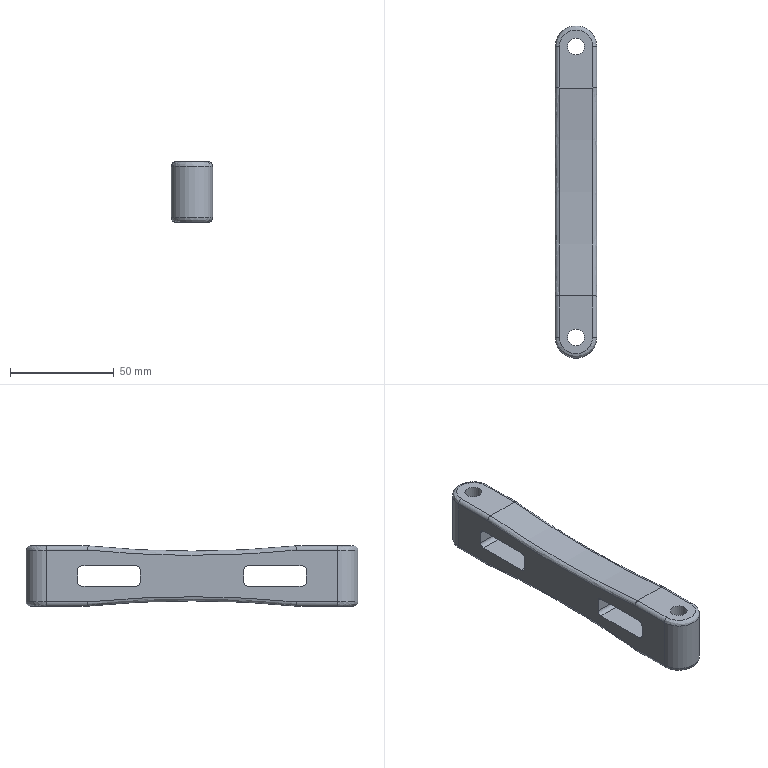Part | STEP file | 1 solid | 44 faces | box 20 x 160 x 29 mm | volume 68270 mm3 | cylinder 22 | plane 14 | spline 8 | commonest cylinder face diameters 4 x16 8 x2 20 x2 1005 x2